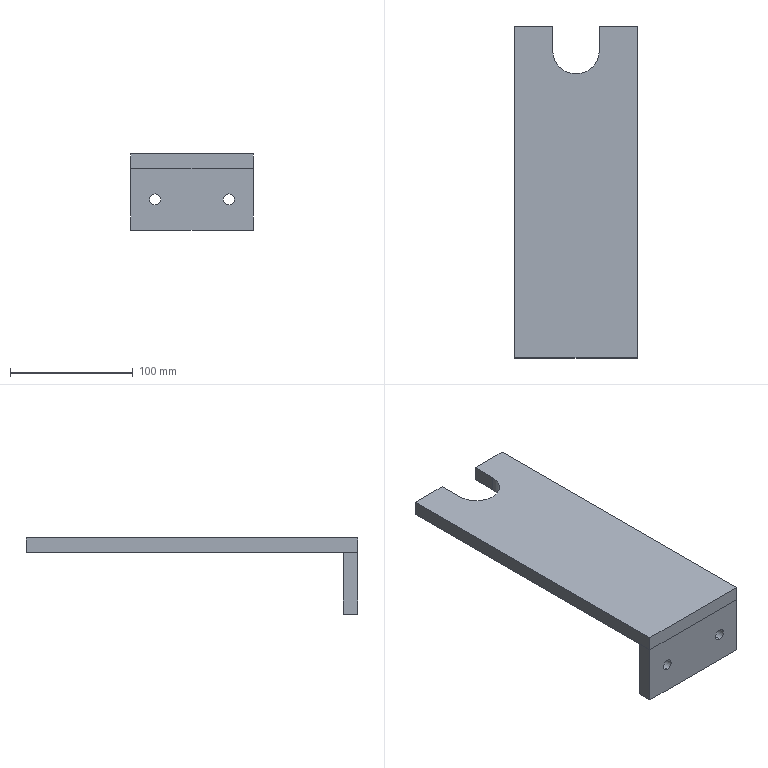Part | STEP file | Feed pipe support plate SGN-6-01 | 2 solids | 32 faces | box 100 x 270 x 62 mm | volume 365504 mm3 | plane 15 | cylinder 9 | cone 8 | commonest cylinder face diameters 4.2 x4 9 x4 38 x1